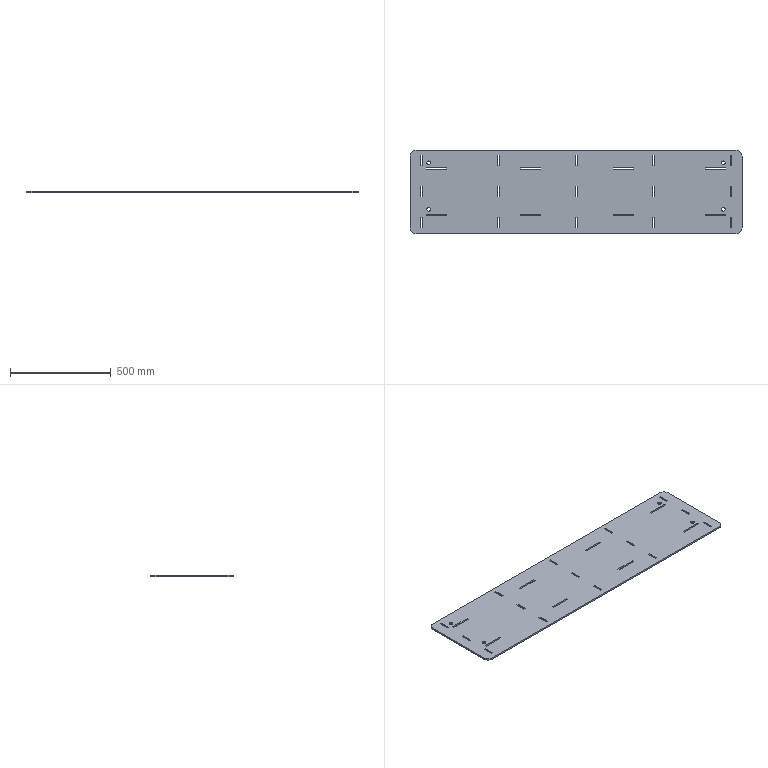Part | SolidWorks | features FlatPattern 1, SMBaseFlange 1, SheetMetal 1 | 1 solid | 110 faces | box 1650 x 415 x 8 mm | volume 5364476 mm3 | plane 98 | cylinder 12 | commonest cylinder face diameters 18 x8 60 x4